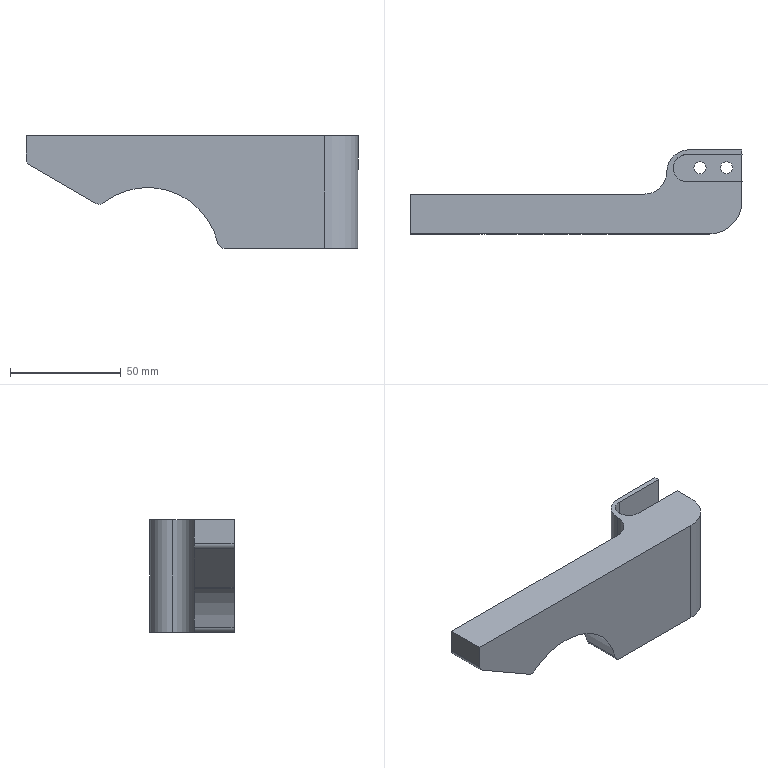NC program | NX | posted with a generic post | part box 150 x 38 x 51 mm
Lines 46 to 1075 of 31037:
(ADAPTIVE_MILLING , TOOL : D12C)
N78 T12 M6
N80 G54
N82 G17 G0 G90 X89.203 Y0.036 S9500 M3
N84 G43 Z30. H12
N86 Z-23.
N88 G94 G1 Z-26. F1000.
N90 X87.519 Y0.629 F3000.
N92 G3 X86.036 Y0.036 R1.218
N94 X85.298 Y-3.27 R9.62
N96 X85.016 Y-14.063 R137.305
N98 G2 X84.974 Y-21.262 R313.
N100 X81.756 Y-26.201 R7.18
N102 X75.529 Y-28.435 R14.662
N104 X66.4 Y-28.949 R69.687
N106 G1 X65.275 Y-28.96
N108 X64. Y-28.969
N110 X62.275 Y-28.976
N112 X60.025 Y-28.981
N114 X56.425 Y-28.985
N116 X48.025 Y-28.986
N118 X-10.7 Y-28.985
N120 X-11.375 Y-28.988
N122 X-12.425 Y-28.989
N124 X-12.875
N126 X-13.775 Y-28.993
N128 X-15.05 Y-28.991
N130 X-15.875 Y-28.994
N132 X-17. Y-28.993
N134 X-17.825 Y-28.995
N136 X-18.95 Y-28.993
N138 X-19.775 Y-28.995
N140 X-20.675 Y-28.994
N142 X-21.8 Y-28.997
N144 X-22.775 Y-28.995
N146 X-23.675 Y-28.997
N148 X-24.575 Y-28.995
N150 X-25.55 Y-28.997
N152 X-26.45 Y-28.995
N154 X-27.35 Y-28.997
N156 X-28.175 Y-28.995
N158 X-29.15 Y-28.996
N160 X-30.125 Y-28.994
N162 X-31.1 Y-28.996
N164 X-31.925 Y-28.995
N166 X-33.05 Y-28.997
N168 X-33.95 Y-28.995
N170 X-34.925 Y-28.997
N172 X-35.75 Y-28.995
N174 X-36.65 Y-28.996
N176 X-37.475 Y-28.995
N178 X-38.675 Y-28.997
N180 X-39.5 Y-28.995
N182 X-40.475 Y-28.997
N184 X-41.225 Y-28.995
N186 X-42.275 Y-28.996
N188 X-43.25 Y-28.994
N190 X-43.925 Y-28.995
N192 X-45.2 Y-28.994
N194 X-45.725
N196 X-46.25 Y-28.995
N198 X-47.45 Y-28.994
N200 X-48.35 Y-28.996
N202 X-49.1 Y-28.995
N204 X-50.375 Y-28.996
N206 X-50.825 Y-28.997
N208 X-51.5 Y-28.995
N210 X-52.85 Y-28.997
N212 X-53.525 Y-28.996
N214 X-54.8 Y-28.997
N216 X-55.25 Y-28.998
N218 X-55.925 Y-28.996
N220 X-57.125 Y-28.997
N222 X-57.725 Y-28.998
N224 X-58.4 Y-28.996
N226 X-59.6 Y-28.997
N228 X-60.5 Y-28.995
N230 X-61.4 Y-28.997
N232 X-62.375 Y-28.995
N234 X-63.275 Y-28.997
N236 X-64.025 Y-28.995
N238 G2 X-77.224 Y-28.968 R754.445
N240 X-82.173 Y-25.766 R7.175
N242 X-84.403 Y-19.694 R14.462
N244 X-84.938 Y-11.168 R62.358
N246 G1 X-84.951 Y-10.193
N248 X-84.961 Y-9.068
N250 X-84.97 Y-7.643
N252 X-84.977 Y-5.843
N254 X-84.982 Y-3.293
N256 X-84.985 Y0.907
N258 X-84.986 Y13.732
N260 Y20.632
N262 X-84.984 Y20.782
N264 X-84.979 Y20.932
N266 X-84.975 Y21.007
N268 X-84.963 Y21.157
N270 G2 X-81.816 Y26.137 R7.109
N272 X-75.755 Y28.394 R14.285
N274 X-66.405 Y28.948 R67.072
N276 G1 X-65.355 Y28.958
N278 X-64.005 Y28.968
N280 X-62.28 Y28.975
N282 X-59.955 Y28.981
N284 X-56.355 Y28.984
N286 X-47.955 Y28.986
N288 X76.695 Y28.983
N290 X76.77 Y28.982
N292 X76.845 Y28.98
N294 X76.995 Y28.973
N296 X77.07 Y28.968
N298 G2 X82.087 Y25.887 R7.047
N300 X84.392 Y19.767 R14.18
N302 X84.935 Y11.317 R60.938
N304 X84.924 Y2.843 R152.035
N306 G3 X84.152 Y-7.099 R142.671
N308 X84.006 Y-17.897 R671.991
N310 G2 X79.627 Y-24.958 R9.157
N312 X72.585 Y-27.363 R17.491
N314 X62.708 Y-27.929 R77.043
N316 G1 X61.583 Y-27.941
N318 X60.158 Y-27.952
N320 X58.508 Y-27.961
N322 X56.333 Y-27.967
N324 X53.258 Y-27.972
N326 X47.708 Y-27.974
N328 X4.583
N330 X-7.342
N332 X-8.017 Y-27.977
N334 X-9.367 Y-27.981
N336 X-10.267 Y-27.982
N338 X-11.017 Y-27.985
N340 X-11.917
N342 X-13.042 Y-27.989
N344 X-14.167 Y-27.988
N346 X-14.917 Y-27.991
N348 X-16.117
N350 X-16.942 Y-27.993
N352 X-17.842 Y-27.992
N354 X-18.892 Y-27.995
N356 X-19.942 Y-27.993
N358 X-20.692 Y-27.995
N360 X-21.892 Y-27.994
N362 X-22.267
N364 X-22.867 Y-27.995
N366 X-23.767 Y-27.994
N368 X-24.292 Y-27.993
N370 X-25.192 Y-27.996
N372 X-25.942 Y-27.995
N374 X-26.917 Y-27.997
N376 X-27.742 Y-27.999
N378 X-28.417 Y-27.997
N380 X-30.367 Y-27.998
N382 X-31.717 Y-28.
N384 X-32.467 Y-27.998
N386 X-33.892
N388 X-34.642 Y-27.999
N390 X-35.467 Y-27.997
N392 X-37.117 Y-28.
N394 X-37.867 Y-27.998
N396 X-38.992
N398 X-39.442
N400 X-40.192 Y-27.997
N402 X-41.242
N404 X-42.367 Y-27.995
N406 X-43.342 Y-27.997
N408 X-44.317 Y-27.994
N410 X-45.292 Y-27.996
N412 X-46.342 Y-27.994
N414 X-47.467 Y-27.997
N416 X-48.292 Y-27.995
N418 X-49.267 Y-27.997
N420 X-49.642
N422 X-50.542 Y-27.996
N424 X-51.442 Y-27.997
N426 X-52.567 Y-27.995
N428 X-53.617 Y-27.998
N430 X-55.042 Y-27.994
N432 X-56.017 Y-27.997
N434 X-56.767 Y-27.996
N436 X-58.192 Y-27.998
N438 X-58.567
N440 X-59.317 Y-27.996
N442 X-60.142 Y-27.997
N444 X-60.517
N446 X-61.342 Y-27.996
N448 X-62.617 Y-27.998
N450 X-63.367 Y-27.996
N452 X-64.342 Y-27.998
N454 X-64.792
N456 X-65.692 Y-27.997
N458 X-66.667 Y-27.998
N460 X-67.567 Y-27.996
N462 X-68.692 Y-27.997
N464 X-69.742 Y-27.995
N466 X-70.792 Y-27.998
N468 X-71.692 Y-27.996
N470 X-72.667 Y-27.997
N472 X-73.342 Y-27.995
N474 X-73.492 Y-27.993
N476 X-73.642 Y-27.988
N478 X-73.791 Y-27.982
N480 X-73.941 Y-27.972
N482 G2 X-80.898 Y-23.682 R9.14
N484 X-83.336 Y-16.731 R17.219
N486 X-83.928 Y-6.781 R75.008
N488 G1 X-83.94 Y-5.656
N490 X-83.951 Y-4.306
N492 X-83.959 Y-2.806
N494 X-83.966 Y-0.781
N496 X-83.971 Y2.069
N498 X-83.974 Y6.869
N500 X-83.975 Y17.369
N502 X-83.972 Y17.519
N504 X-83.967 Y17.669
N506 X-83.961 Y17.819
N508 X-83.951 Y17.968
N510 G2 X-79.524 Y24.998 R9.158
N512 X-72.545 Y27.366 R17.665
N514 X-62.968 Y27.924 R76.484
N516 G1 X-61.918 Y27.937
N518 X-60.643 Y27.948
N520 X-59.143 Y27.957
N522 X-57.268 Y27.964
N524 X-54.718 Y27.969
N526 X-50.668 Y27.973
N528 X-40.468 Y27.974
N530 X73.307 Y27.972
N532 X73.532 Y27.969
N534 X73.682 Y27.964
N536 X73.832 Y27.956
N538 X73.982 Y27.947
N540 G2 X80.882 Y23.697 R9.11
N542 X83.335 Y16.751 R17.193
N544 X83.604 Y0.287 R75.487
N546 G3 X83.034 Y-15.225 R238.426
N548 G2 X80.62 Y-21.48 R10.4
N550 X76.415 Y-25.031 R6.623
N552 X67.442 Y-26.667 R33.231
N554 X51.548 Y-26.958 R274.604
N556 G1 X47.423 Y-26.962
N558 X38.273 Y-26.963
N560 X-4.027 Y-26.962
N562 X-4.777 Y-26.966
N564 X-5.902 Y-26.969
N566 X-6.877
N568 X-7.702 Y-26.974
N570 X-8.677 Y-26.976
N572 X-9.127 Y-26.977
N574 X-9.877 Y-26.98
N576 X-10.852 Y-26.981
N578 X-11.227
N580 X-12.052 Y-26.984
N582 X-13.177 Y-26.985
N584 X-14.077 Y-26.988
N586 X-14.977
N588 X-15.877 Y-26.99
N590 X-16.927
N592 X-17.752 Y-26.992
N594 X-19.027 Y-26.991
N596 X-19.852 Y-26.993
N598 X-21.052 Y-26.991
N600 X-22.027 Y-26.994
N602 X-22.852 Y-26.993
N604 X-23.902 Y-26.996
N606 X-24.277
N608 X-25.327 Y-26.995
N610 X-26.227 Y-26.997
N612 X-27.277 Y-26.995
N614 X-28.027 Y-26.997
N616 X-29.152 Y-26.996
N618 X-29.752 Y-26.995
N620 X-30.727 Y-26.998
N622 X-31.402 Y-26.997
N624 X-32.902 Y-27.
N626 X-33.727 Y-27.002
N628 X-34.702 Y-26.999
N630 X-35.527 Y-27.
N632 X-36.877 Y-26.997
N634 X-37.852 Y-26.999
N636 X-39.127 Y-26.996
N638 X-40.102 Y-26.997
N640 X-41.302 Y-26.995
N642 X-42.202 Y-26.996
N644 X-43.252 Y-26.994
N646 X-44.452 Y-26.997
N648 X-45.427 Y-26.995
N650 X-46.327 Y-26.997
N652 X-47.452 Y-26.995
N654 X-48.277 Y-26.997
N656 X-49.327 Y-26.995
N658 X-50.452 Y-26.998
N660 X-51.802 Y-26.994
N662 X-52.927 Y-26.997
N664 X-53.902 Y-26.995
N666 X-55.027 Y-26.998
N668 G2 X-71.451 Y-26.961 R912.148
N670 X-79.992 Y-21.503 R10.559
N672 X-82.343 Y-14.04 R20.138
N674 X-82.915 Y-3.488 R88.971
N676 X-82.925 Y15.561 R712.563
N678 X-80.673 Y21.341 R10.267
N680 X-76.494 Y25.002 R6.504
N682 X-67.6 Y26.653 R32.741
N684 X-53.506 Y26.953 R231.267
N686 G1 X-50.431 Y26.959
N688 X-45.556 Y26.962
N690 X-30.031
N692 X70.394 Y26.96
N694 X70.619 Y26.958
N696 X70.769 Y26.956
N698 G2 X80.029 Y21.425 R10.543
N700 X82.343 Y14.028 R20.208
N702 X82.627 Y1.453 R63.307
N704 G3 X82.064 Y-13.085 R402.459
N706 G2 X81.164 Y-17.325 R15.615
N708 X80.972 Y-20.435 R17.594
N710 G1 X80.576 Y-21.568
N712 G3 X81.15 Y-18.965 R7.23
N714 G1 Y-17.454
N716 G3 X81.5 Y-10.865 R437.086
N718 G2 X82.131 Y3.971 R830.594
N720 G3 X81.405 Y15.324 R50.482
N722 X78.52 Y21.928 R15.343
N724 X71.963 Y25.701 R11.001
N726 X64.574 Y26.309 R40.353
N728 G1 X63.824 Y26.32
N730 X62.774 Y26.332
N732 X61.724 Y26.339
N734 X60.224 Y26.346
N736 X58.049 Y26.35
N738 X54.224 Y26.353
N740 X33.149 Y26.355
N742 X-52.051 Y26.357
N744 X-57.151 Y26.334
N746 G3 X-69.36 Y25.838 R124.61
N748 X-73.447 Y25.15 R47.801
N750 X-76.44 Y24.971 R14.602
N752 G1 X-77.61 Y24.561
N754 G2 X-74.964 Y25.15 R7.291
N756 G1 X-73.447
N758 G3 X-58.524 Y25.289 R377.149
N760 G1 X-57.249 Y25.304
N762 X-55.599 Y25.318
N764 X-53.8 Y25.33
N766 X-52. Y25.339
N768 X-50.2 Y25.344
N770 X-48.1 Y25.345
N772 X59.6 Y25.342
N774 X60.575 Y25.336
N776 X61.925 Y25.323
N778 G2 X69.853 Y24.856 R52.121
N780 X78.823 Y18. R11.781
N782 X80.83 Y9.964 R23.954
N784 X81.027 Y5.878 R73.154
N786 G1 X81.149 Y4.021
N788 X81.15 Y3.979
N790 Y-17.171
N792 Y3.979
N794 X81.149 Y4.021
N796 X80.972 Y6.719
N798 X80.961 Y6.801
N800 G3 X79.558 Y13.692 R161.545
N802 X76.06 Y20.401 R14.977
N804 X69.322 Y23.942 R13.065
N806 X64.968 Y24.53 R32.354
N808 G1 X62.801 Y24.961
N810 X62.719 Y24.972
N812 X60.021 Y25.149
N814 X59.979 Y25.15
N816 X-63.996
N818 G2 X-64.828 Y27.215 R1.201
N820 X-64.19 Y27.558 Z-25.97 R1.663
N822 G1 X-62.625 Y28.139 Z-25.9
N824 X-60.457 Y28.935
N826 X-60.177 Y28.968
N828 X62.268 Y29.206
N830 G2 X63.445 Y28.252 R1.208
N832 G1 X63.518 Y27.902
N834 X64.009 Y25.553 Z-26.
N836 G3 X64.968 Y24.53 R1.222
N838 G1 X65.433 Y24.437
N840 X65.513 Y24.416
N842 G2 X71.356 Y22.106 R36.87
N844 X76.234 Y17.497 R13.318
N846 G1 X76.752 Y16.906
N848 X76.802 Y16.841
N850 X78.293 Y14.609
N852 X78.335 Y14.538
N854 X79.522 Y12.131
N856 X79.553 Y12.055
N858 X80.416 Y9.513
N860 X80.437 Y9.433
N862 X79.522 Y12.131
N864 X78.293 Y14.609
N866 X76.752 Y16.906
N868 X74.983 Y18.924
N870 X74.924 Y18.983
N872 X72.906 Y20.752
N874 X72.841 Y20.802
N876 X70.609 Y22.293
N878 X70.538 Y22.335
N880 X68.131 Y23.522
N882 G2 X68.698 Y25.797 R1.201
N884 G1 X69.884 Y25.616 Z-25.95
N886 X71.066 Y25.41 Z-25.9
N888 X72.057 Y25.249
N890 X73.044 Y25.065
N892 X73.347 Y24.919
N894 X74.593 Y24.089
N896 X75.83 Y23.244
N898 G2 X79.142 Y20.036 R17.57
N900 X84.49 Y6.926 R25.143
N902 G1 X84.606 Y5.585
N904 X84.671 Y4.242
N906 X85.313 Y-21.693
N908 G2 X84.174 Y-23.822 R2.462
N910 G1 X83.512 Y-24.248
N912 X82.836 Y-24.652
N914 G2 X82.148 Y-24.74 R1.405
N916 G1 X79.752 Y-24.598 Z-26.
N918 X78.832 Y-24.541
N920 X77.91 Y-24.5
N922 X77.601 Y-24.564
N924 G2 X74.14 Y-25.15 R7.644
N926 X53.987 Y-25.933 R225.901
N928 G1 X51.737 Y-25.941
N930 X48.812 Y-25.946
N932 X44.387 Y-25.95
N934 X34.562 Y-25.952
N936 X-0.688 Y-25.951
N938 X-1.588 Y-25.956
N940 X-2.713 Y-25.958
N942 X-3.538 Y-25.962
N944 X-4.363 Y-25.963
N946 X-5.263 Y-25.967
N948 X-6.313 Y-25.968
N950 X-7.063 Y-25.972
N952 X-8.038 Y-25.973
N954 X-8.863 Y-25.976
N956 X-9.238 Y-25.977
N958 X-10.138 Y-25.978
N960 X-11.263 Y-25.982
N962 X-12.163
N964 X-13.138 Y-25.986
N966 X-14.038 Y-25.985
N968 X-14.938 Y-25.988
N970 X-15.913
N972 X-16.963 Y-25.991
N974 X-17.788 Y-25.99
N976 X-18.913 Y-25.992
N978 X-19.288 Y-25.993
N980 X-20.188 Y-25.991
N982 X-21.088 Y-25.993
N984 X-22.138
N986 X-22.513 Y-25.992
N988 X-23.338 Y-25.995
N990 X-24.463 Y-25.993
N992 X-25.363 Y-25.996
N994 X-26.263 Y-25.995
N996 X-27.538 Y-25.997
N998 X-28.363 Y-25.996
N1000 X-29.263 Y-25.998
N1002 X-29.788 Y-25.999
N1004 X-30.388
N1006 X-31.438 Y-26.
N1008 X-32.188 Y-25.999
N1010 X-33.088 Y-26.
N1012 X-33.988 Y-25.999
N1014 X-35.038 Y-26.
N1016 X-36.013 Y-25.998
N1018 X-37.138 Y-25.999
N1020 X-38.188 Y-25.996
N1022 X-39.013 Y-25.997
N1024 X-40.138 Y-25.995
N1026 X-40.588
N1028 X-41.338 Y-25.996
N1030 X-42.538 Y-25.995
N1032 X-43.438 Y-25.997
N1034 X-44.488 Y-25.995
N1036 X-45.313 Y-25.996
N1038 X-46.513 Y-25.995
N1040 X-47.413 Y-25.996
N1042 X-48.388 Y-25.995
N1044 X-49.288 Y-25.996
N1046 X-49.738 Y-25.997
N1048 X-50.788 Y-25.995
N1050 X-51.913 Y-25.997
N1052 X-52.963 Y-25.995
N1054 X-54.163 Y-25.998
N1056 X-54.988 Y-25.996
N1058 X-56.188 Y-25.997
N1060 X-57.163 Y-25.996
N1062 X-58.213 Y-25.998
N1064 X-59.413 Y-25.995
N1066 X-60.388 Y-25.998
N1068 X-61.363 Y-25.996
N1070 X-62.413 Y-25.998
N1072 X-63.538 Y-25.996
N1074 X-64.363 Y-25.998
N1076 X-65.563 Y-25.996
N1078 G2 X-70.801 Y-25.772 R31.677
N1080 X-79.03 Y-19.615 R11.592
N1082 X-81.339 Y-11.744 R22.4
N1084 X-81.901 Y-0.889 R98.095
N1086 X-81.906 Y13.36 R427.789
N1088 X-81.15 Y17.126 R17.724
N1090 X-80.979 Y20.409 R17.086
N1092 G1 X-80.611 Y21.472
N1094 G3 X-81.15 Y18.934 R7.107
N1096 G1 Y17.126
N1098 G3 X-81.091 Y-7.242 R323.116
N1100 X-79.79 Y-15.671 R35.84
N1102 X-75.492 Y-22.392 R13.486
N1104 X-69.019 Y-24.964 R13.125
N1106 X-61.161 Y-25.369 R62.56
N1108 G1 X-59.886 Y-25.378
N1110 X-58.611 Y-25.383
N1112 X-57.336 Y-25.386
N1114 X-56.736 Y-25.389
N1116 X-53.061 Y-25.391
N1118 X-52.686
N1120 X-52.086 Y-25.392
N1122 X-51.111 Y-25.391
N1124 X-50.061 Y-25.395
N1126 X-49.011 Y-25.393
N1128 X-47.661 Y-25.396
N1130 X-47.211
N1132 X-45.486 Y-25.398
N1134 X-44.736 Y-25.396
N1136 X-44.286
N1138 X-42.561 Y-25.393
N1140 X-41.586 Y-25.396
N1142 X-40.461 Y-25.395
N1144 X-40.011
N1146 X-36.411
N1148 X-32.811 Y-25.398
N1150 X-31.836 Y-25.4
N1152 X-31.386 Y-25.399
N1154 X-29.811 Y-25.4
N1156 X-28.611 Y-25.397
N1158 X-27.861 Y-25.398
N1160 X-27.336 Y-25.396
N1162 X-25.761 Y-25.398
N1164 X-24.861 Y-25.395
N1166 X-24.336
N1168 X-23.736 Y-25.394
N1170 X-23.211
N1172 X-22.386 Y-25.392
N1174 X-21.936
N1176 X-20.811 Y-25.39
N1178 X-20.286 Y-25.391
N1180 X-19.836 Y-25.39
N1182 X-19.311 Y-25.391
N1184 X-18.786 Y-25.39
N1186 X-17.736 Y-25.391
N1188 X-16.236 Y-25.387
N1190 X-15.411 Y-25.388
N1192 X-14.811 Y-25.385
N1194 X-13.686 Y-25.386
N1196 X-12.861 Y-25.383
N1198 X-11.661
N1200 X-11.136 Y-25.381
N1202 X-9.411 Y-25.379
N1204 X-8.961 Y-25.378
N1206 X-7.911 Y-25.376
N1208 X-6.786 Y-25.37
N1210 X-6.261 Y-25.369
N1212 X-4.986 Y-25.363
N1214 X-4.086
N1216 X-3.336 Y-25.359
N1218 X1.239 Y-25.358
N1220 X16.614
N1222 X16.914 Y-25.356
N1224 X40.314 Y-25.357
N1226 X40.689 Y-25.355
N1228 X43.539
N1230 X43.914 Y-25.354
N1232 G3 X64.385 Y-25.15 R657.847
N1234 G1 X74.21
N1236 X51.025
N1238 X50.975 Y-25.148
N1240 G2 X46.796 Y-24.685 R37.976
N1242 G3 X37.729 Y-24.386 R102.385
N1244 G1 X36.079 Y-24.379
N1246 X33.754 Y-24.373
N1248 X30.079 Y-24.37
N1250 X20.854 Y-24.368
N1252 X-0.671 Y-24.369
N1254 X-8.246 Y-24.37
N1256 X-8.846 Y-24.373
N1258 X-10.271 Y-24.376
N1260 X-11.621 Y-24.377
N1262 X-12.446 Y-24.38
N1264 X-13.271 Y-24.381
N1266 X-13.721 Y-24.382
N1268 X-14.546 Y-24.385
N1270 X-15.446
N1272 X-15.821
N1274 X-16.571 Y-24.387
N1276 X-17.696
N1278 X-18.596 Y-24.389
N1280 X-19.646 Y-24.388
N1282 X-20.396 Y-24.391
N1284 X-21.371 Y-24.39
N1286 X-21.746
N1288 X-22.721 Y-24.394
N1290 X-24.146 Y-24.392
N1292 X-24.821 Y-24.394
N1294 X-26.171
N1296 X-26.621 Y-24.395
N1298 X-27.296 Y-24.397
N1300 X-28.346 Y-24.396
N1302 X-29.171 Y-24.398
N1304 X-30.146 Y-24.397
N1306 X-30.821 Y-24.398
N1308 X-31.796 Y-24.396
N1310 X-32.321
N1312 X-32.996 Y-24.397
N1314 X-33.821 Y-24.396
N1316 X-35.021 Y-24.397
N1318 X-35.696 Y-24.396
N1320 X-36.746 Y-24.397
N1322 X-37.271
N1324 X-37.796 Y-24.395
N1326 X-38.846 Y-24.397
N1328 X-39.746 Y-24.395
N1330 X-40.346 Y-24.396
N1332 X-41.171 Y-24.398
N1334 X-41.845 Y-24.397
N1336 X-43.495 Y-24.398
N1338 X-44.095 Y-24.399
N1340 X-44.77 Y-24.397
N1342 X-45.745
N1344 X-46.42 Y-24.396
N1346 X-47.545
N1348 X-48.22 Y-24.395
N1350 X-49.27
N1352 X-49.645
N1354 X-50.395 Y-24.393
N1356 X-51.445
N1358 X-52.27 Y-24.391
N1360 X-53.32 Y-24.393
N1362 X-54.22 Y-24.39
N1364 X-55.495
N1366 X-57.37 Y-24.38
N1368 G2 X-66.886 Y-24.074 R100.081
N1370 X-74.01 Y-21.38 R13.384
N1372 X-78.611 Y-14.32 R14.601
N1374 X-80.041 Y-5.609 R36.145
N1376 G3 X-80.237 Y-2.242 R50.216
N1378 G2 X-81.002 Y-0.306 R10.588
N1380 G1 X-81.146 Y0.955
N1382 X-81.15 Y1.026
N1384 Y16.701
N1386 X-81.146 Y0.955
N1388 G3 X-80.561 Y-1.608 R7.129
N1390 G1 X-80.325 Y-2.012
N1392 G2 X-79.778 Y-3.948 R5.4
N1394 G3 X-78.721 Y-11.068 R123.889
N1396 X-75.573 Y-18.373 R17.53
N1398 X-68.017 Y-22.926 R13.069
N1400 X-60.269 Y-23.704 R39.442
N1402 X-39.345 Y-23.796 R976.026
N1404 G1 X-38.145 Y-23.794
N1406 X-37.245 Y-23.796
N1408 X-36.195 Y-23.794
N1410 X-35.295 Y-23.797
N1412 X-34.395 Y-23.795
N1414 X-33.27 Y-23.798
N1416 X-32.37 Y-23.796
N1418 X-31.62 Y-23.798
N1420 X-31.095 Y-23.797
N1422 X-30.27 Y-23.799
N1424 X-28.77 Y-23.795
N1426 X-27.87 Y-23.796
N1428 X-26.445 Y-23.793
N1430 X-25.02 Y-23.795
N1432 X-24.345 Y-23.793
N1434 X-22.845 Y-23.794
N1436 X-21.87 Y-23.791
N1438 X-20.895 Y-23.792
N1440 X-19.92 Y-23.789
N1442 X-19.095 Y-23.787
N1444 X-18.645
N1446 X-18.345 Y-23.786
N1448 X-17.07 Y-23.788
N1450 X-16.17 Y-23.784
N1452 X-14.97 Y-23.785
N1454 X-13.995 Y-23.781
N1456 X-13.245 Y-23.782
N1458 X-12.72 Y-23.78
N1460 X-12.045
N1462 X-10.32 Y-23.774
N1464 X-8.445 Y-23.775
N1466 X-8.07 Y-23.773
N1468 X-6.27 Y-23.774
N1470 X-5.895 Y-23.773
N1472 X-3.945 Y-23.774
N1474 X-3.57 Y-23.772
N1476 X-1.62 Y-23.774
N1478 X-1.245 Y-23.772
N1480 X0.78 Y-23.773
N1482 X1.155 Y-23.772
N1484 X3.33 Y-23.773
N1486 X3.705 Y-23.772
N1488 X5.88 Y-23.773
N1490 X6.255 Y-23.772
N1492 X8.58 Y-23.773
N1494 X8.955 Y-23.771
N1496 X11.355 Y-23.773
N1498 X11.73 Y-23.771
N1500 X14.28 Y-23.773
N1502 X14.655 Y-23.771
N1504 X17.355 Y-23.773
N1506 X17.73 Y-23.772
N1508 X20.58 Y-23.773
N1510 X20.955 Y-23.772
N1512 G2 X42.854 Y-23.878 R959.946
N1514 X45.25 Y-24.045 R17.211
N1516 G1 X45.964 Y-24.341
N1518 X46.058 Y-24.371
N1520 X48.318 Y-24.914
N1522 X46.058 Y-24.371
N1524 X45.964 Y-24.341
N1526 X45.25 Y-24.045
N1528 G3 X41.031 Y-23.084 R12.285
N1530 X29.338 Y-22.794 R155.998
N1532 G1 X26.788 Y-22.789
N1534 X20.788 Y-22.784
N1536 X14.413 Y-22.782
N1538 X12.988
N1540 X12.388 Y-22.78
N1542 X10.363 Y-22.776
N1544 X8.413
N1546 X7.513 Y-22.777
N1548 X6.838 Y-22.776
N1550 X5.413 Y-22.775
N1552 X4.588 Y-22.776
N1554 X3.688 Y-22.774
N1556 X2.863
N1558 X1.813 Y-22.773
N1560 X0.913 Y-22.774
N1562 X-0.212 Y-22.772
N1564 X-0.962 Y-22.773
N1566 X-1.937 Y-22.772
N1568 X-2.462
N1570 X-3.212 Y-22.774
N1572 X-3.962 Y-22.773
N1574 X-4.862 Y-22.774
N1576 X-5.387 Y-22.775
N1578 X-6.137 Y-22.774
N1580 X-7.112 Y-22.775
N1582 X-7.712 Y-22.774
N1584 X-8.762 Y-22.777
N1586 X-9.887
N1588 X-10.862 Y-22.779
N1590 X-11.612
N1592 X-12.512 Y-22.781
N1594 X-13.562
N1596 X-14.237 Y-22.783
N1598 X-15.362
N1600 X-15.887 Y-22.784
N1602 X-16.637 Y-22.786
N1604 X-17.237
N1606 X-18.437 Y-22.789
N1608 X-19.262 Y-22.792
N1610 X-20.237 Y-22.79
N1612 X-21.062 Y-22.792
N1614 X-21.812
N1616 X-22.712 Y-22.793
N1618 X-23.687 Y-22.792
N1620 X-24.737 Y-22.795
N1622 X-25.787 Y-22.793
N1624 X-26.762 Y-22.796
N1626 X-27.812 Y-22.794
N1628 X-28.562 Y-22.796
N1630 X-29.462 Y-22.795
N1632 X-29.837
N1634 X-30.662 Y-22.797
N1636 X-31.562 Y-22.795
N1638 X-32.537 Y-22.797
N1640 X-33.287 Y-22.795
N1642 X-34.412 Y-22.797
N1644 X-35.462 Y-22.794
N1646 X-36.212 Y-22.796
N1648 X-37.412 Y-22.794
N1650 X-37.862
N1652 X-38.387 Y-22.795
N1654 G2 X-60.361 Y-22.663 R859.95
N1656 X-67.774 Y-21.671 R29.712
N1658 X-76.095 Y-14.297 R13.253
N1660 X-78.194 Y-6.964 R29.292
N1662 G3 X-78.86 Y-3.889 R30.668
N1664 X-79.843 Y-2.779 R6.598
N1666 G1 X-80.282 Y-2.081
N1668 X-79.843 Y-2.779
N1670 X-79.755 Y-2.889
N1672 X-79.066 Y-3.577
N1674 G2 X-78.218 Y-5.227 R3.832
N1676 G3 X-76.67 Y-10.789 R723.715
N1678 X-72.713 Y-17.592 R16.185
N1680 X-65.237 Y-21.334 R14.928
N1682 X-56.659 Y-22.104 R47.173
N1684 X-35.735 Y-22.191 R974.906
N1686 G1 X-34.835 Y-22.194
N1688 X-34.16 Y-22.193
N1690 X-33.035 Y-22.196
N1692 X-32.285 Y-22.194
N1694 X-31.835 Y-22.195
N1696 X-28.16 Y-22.191
N1698 X-24.485 Y-22.192
N1700 X-22.985 Y-22.194
N1702 X-22.535 Y-22.192
N1704 X-21.935 Y-22.193
N1706 X-20.66 Y-22.19
N1708 X-20.21
N1710 X-19.61 Y-22.188
N1712 X-18.935 Y-22.189
N1714 X-17.885 Y-22.185
N1716 X-16.76 Y-22.187
N1718 X-15.71 Y-22.183
N1720 X-14.81 Y-22.184
N1722 X-13.76 Y-22.181
N1724 X-12.185 Y-22.177
N1726 X-11.36 Y-22.179
N1728 X-10.835 Y-22.178
N1730 X-7.235 Y-22.179
N1732 X-3.635 Y-22.175
N1734 X-1.985 Y-22.173
N1736 X-1.385 Y-22.174
N1738 X-0.41 Y-22.172
N1740 X0.64 Y-22.175
N1742 X1.39 Y-22.173
N1744 X2.14 Y-22.175
N1746 X2.59 Y-22.174
N1748 X3.04 Y-22.175
N1750 X3.79 Y-22.174
N1752 X5.215 Y-22.177
N1754 X6.64 Y-22.174
N1756 X7.315 Y-22.176
N1758 X7.84 Y-22.175
N1760 X10.99 Y-22.183
N1762 X11.74 Y-22.181
N1764 X12.34 Y-22.183
N1766 X13.165 Y-22.181
N1768 X13.84 Y-22.183
N1770 X14.59 Y-22.181
N1772 X15.265 Y-22.183
N1774 X15.94 Y-22.181
N1776 X16.69 Y-22.183
N1778 X17.365 Y-22.182
N1780 X18.115 Y-22.184
N1782 X18.715 Y-22.183
N1784 X19.54 Y-22.185
N1786 X20.065 Y-22.184
N1788 X20.89 Y-22.185
N1790 X21.415 Y-22.184
N1792 X22.39 Y-22.187
N1794 X22.915 Y-22.186
N1796 X24.04 Y-22.188
N1798 X24.49
N1800 G2 X39.037 Y-22.384 R322.474
N1802 X42.752 Y-22.841 R18.77
N1804 G3 X44.545 Y-23.753 R9.024
N1806 G1 X43.714 Y-23.409
N1808 X43.626 Y-23.364
N1810 X42.821 Y-22.871
N1812 G3 X39.505 Y-21.761 R8.069
N1814 X31.352 Y-21.258 R61.96
N1816 X12.002 Y-21.187 R995.343
N1818 G1 X11.327 Y-21.184
N1820 X10.052 Y-21.182
N1822 X8.402 Y-21.183
N1824 X7.727 Y-21.181
N1826 X5.927 Y-21.179
N1828 X3.902 Y-21.181
N1830 X3.227 Y-21.179
N1832 X1.502 Y-21.177
N1834 X-0.298 Y-21.179
N1836 X-0.748
N1838 X-1.348 Y-21.177
N1840 X-2.023 Y-21.178
N1842 X-2.623 Y-21.179
N1844 X-3.373 Y-21.178
N1846 X-4.648 Y-21.18
N1848 X-5.098
N1850 X-5.773 Y-21.179
N1852 X-6.973 Y-21.181
N1854 X-7.348
N1856 X-8.023 Y-21.18
N1858 X-9.298 Y-21.181
N1860 X-10.498 Y-21.183
N1862 X-11.098
N1864 X-13.198 Y-21.184
N1866 X-15.073 Y-21.188
N1868 X-15.673 Y-21.19
N1870 X-16.648 Y-21.188
N1872 X-18.298 Y-21.192
N1874 X-19.273 Y-21.19
N1876 X-20.248 Y-21.193
N1878 X-21.298 Y-21.191
N1880 X-21.973 Y-21.192
N1882 X-23.248 Y-21.19
N1884 X-23.698
N1886 X-24.673 Y-21.192
N1888 X-25.573 Y-21.191
N1890 X-26.623 Y-21.192
N1892 X-27.298
N1894 X-28.423 Y-21.194
N1896 X-28.948
N1898 X-29.548 Y-21.193
N1900 X-30.373 Y-21.194
N1902 X-31.498 Y-21.193
N1904 X-32.173 Y-21.194
N1906 X-33.298 Y-21.192
N1908 X-34.123 Y-21.193
N1910 X-35.023 Y-21.191
N1912 X-35.923
N1914 X-36.898 Y-21.19
N1916 G2 X-57.446 Y-21.047 R751.289
N1918 X-65.242 Y-20.064 R34.122
N1920 X-74.405 Y-12.442 R14.207
N1922 X-76.645 Y-6.721 R45.77
N1924 G3 X-77.616 Y-4.619 R7.603
N1926 X-78.881 Y-3.761 R19.136
N1928 G1 X-78.934 Y-3.708
N1930 X-78.881 Y-3.761
N1932 X-78.771 Y-3.848
N1934 X-77.792 Y-4.463
N1936 G2 X-76.716 Y-5.786 R3.168
N1938 X-74.595 Y-10.504 R119.918
N1940 G3 X-69.248 Y-17.137 R15.994
N1942 X-61.565 Y-19.945 R18.402
N1944 X-52.14 Y-20.525 R70.804
N1946 X-32.941 Y-20.592 R977.359
N1948 G1 X-32.566 Y-20.593
N1950 X-32.041
N1952 X-31.516 Y-20.594
N1954 X-29.641 Y-20.59
N1956 X-28.816 Y-20.592
N1958 X-28.366 Y-20.591
N1960 X-26.941 Y-20.594
N1962 X-26.416 Y-20.593
N1964 X-22.816 Y-20.594
N1966 X-19.216 Y-20.591
N1968 X-15.691 Y-20.584
N1970 X-15.166 Y-20.585
N1972 X-14.341 Y-20.583
N1974 X-13.516 Y-20.584
N1976 X-13.216 Y-20.583
N1978 X-12.691 Y-20.584
N1980 X-12.166 Y-20.583
N1982 X-11.641 Y-20.584
N1984 X-11.041 Y-20.582
N1986 X-9.241 Y-20.584
N1988 X-8.566 Y-20.582
N1990 X-7.066 Y-20.583
N1992 X-6.391 Y-20.581
N1994 X-4.816 Y-20.582
N1996 X-3.916 Y-20.579
N1998 X-2.941 Y-20.581
N2000 X-0.241
N2002 X2.009 Y-20.579
N2004 X2.459 Y-20.58
N2006 X3.434 Y-20.578
N2008 X4.334 Y-20.58
N2010 X4.784 Y-20.579
N2012 X6.359 Y-20.583
N2014 X7.634 Y-20.581
N2016 X10.409 Y-20.587
N2018 X10.784
N2020 X11.834 Y-20.59
N2022 X12.434 Y-20.591
N2024 X13.559 Y-20.589
N2026 X14.159 Y-20.591
N2028 X14.984 Y-20.59
N2030 X15.809 Y-20.592
N2032 X16.409 Y-20.591
N2034 G2 X34.482 Y-20.765 R551.018
N2036 X40.793 Y-21.561 R28.123
N2038 X41.55 Y-22.092 R3.098
N2040 G1 X42.381 Y-22.601
N2042 X41.55 Y-22.092
N2044 X41.47 Y-22.033
N2046 X41.093 Y-21.712
N2048 G3 X38.385 Y-20.497 R5.987
N2050 X30.711 Y-19.735 R40.312
N2052 X8.887 Y-19.59 R944.708
N2054 G1 X7.237 Y-19.587
N2056 X5.587
N2058 X4.912 Y-19.584
N2060 X3.862
N2062 X3.187 Y-19.585
N2064 X2.362 Y-19.583
N2066 X1.162 Y-19.584
N2068 X0.262 Y-19.582
N2070 X-0.563
N2072 X-1.388 Y-19.581
N2074 X-2.363 Y-19.582
N2076 X-3.338 Y-19.581
N2078 X-4.163 Y-19.582
N2080 X-5.288 Y-19.581
N2082 X-5.738
N2084 X-6.563 Y-19.583
N2086 X-7.388 Y-19.582
N2088 X-8.588 Y-19.584
N2090 X-9.113 Y-19.585
N2092 X-10.163 Y-19.582
N2094 X-10.838 Y-19.583
N2096 X-12.113 Y-19.582
N2098 X-12.638
N2100 X-13.463 Y-19.585
N2102 X-14.363 Y-19.584
N2104 X-15.338 Y-19.586
N2106 X-16.313 Y-19.585
N2108 X-17.063 Y-19.588
N2110 X-18.188
N2112 X-18.638
N2114 X-19.313 Y-19.59
N2116 X-20.438
N2118 X-20.813
N2120 X-21.713 Y-19.592
N2122 X-22.538 Y-19.591
N2124 X-23.813 Y-19.594
N2126 X-24.563 Y-19.593
N2128 X-25.763 Y-19.594
N2130 X-26.213